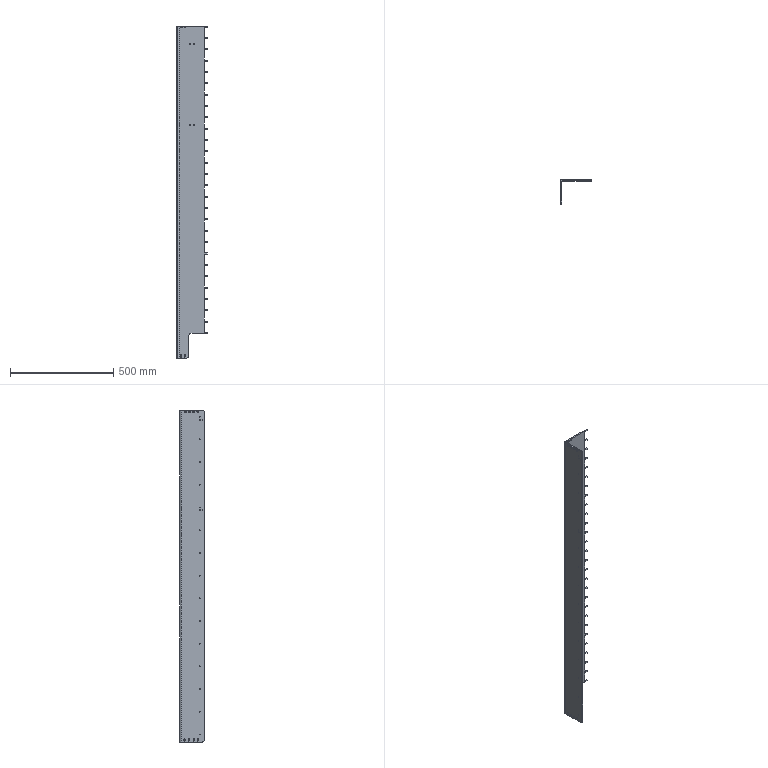Part | SolidWorks | features HoleWzd 7, Fillet 2, Cut 1, Extrusion 1, ICE 1, LPattern 1, MoveFace 1 | 1 solid | 224 faces | box 150 x 120 x 1609 mm | volume 2357171 mm3 | plane 130 | cylinder 82 | cone 12 | commonest cylinder face diameters 4.2 x38 5.8 x18 5.5 x12 5 x8 20 x4 16 x2